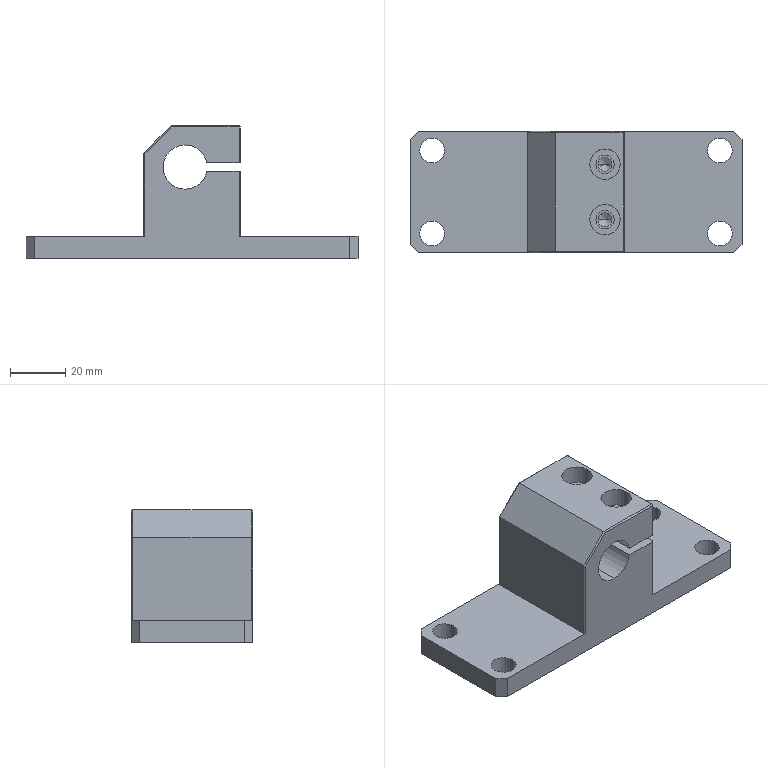Part | NX | features BREP 1 | 1 solid | 60 faces | box 120 x 44 x 48 mm | volume 86553 mm3 | plane 33 | cylinder 23 | cone 4 | commonest cylinder face diameters 9 x8 5 x4 6.6 x4 11 x4 16 x3